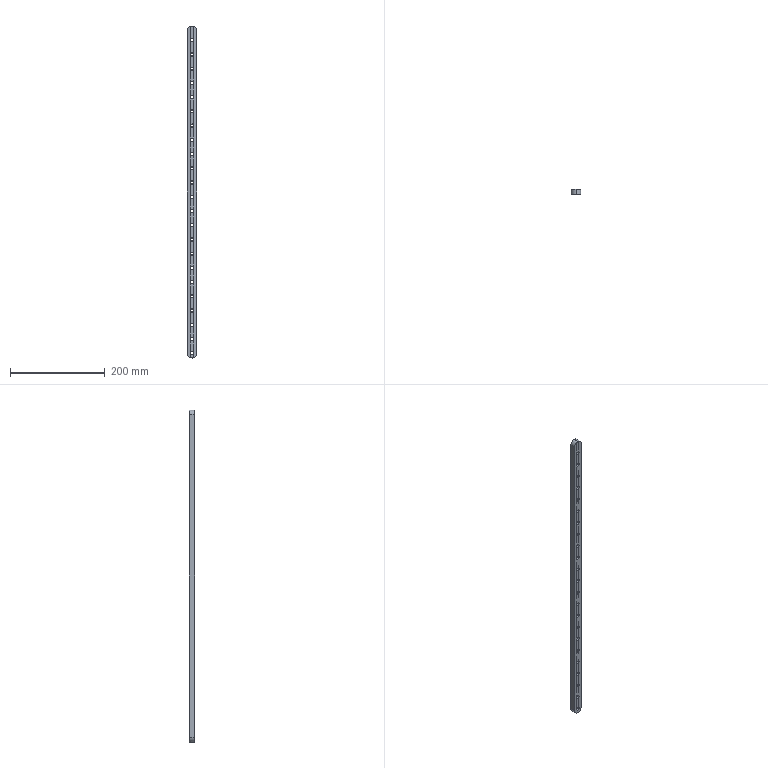Part | SolidWorks | features Extrusion 1, Fillet 1, HoleWzd 1, ICE 1, LPattern 1, MirrorPattern 1 | 1 solid | 79 faces | box 20 x 11 x 700 mm | volume 140963 mm3 | cylinder 50 | plane 29 | commonest cylinder face diameters 6.8 x46 20 x4